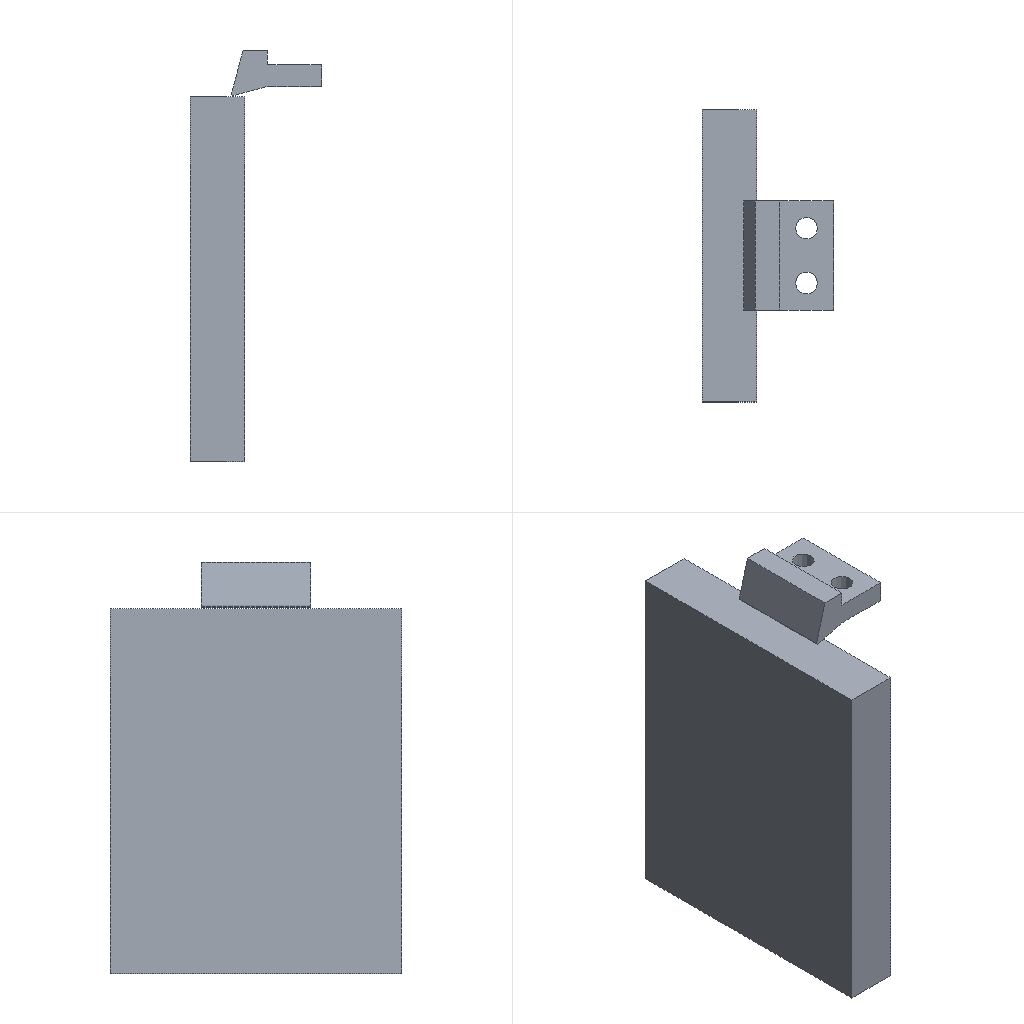Simulation study | abaqus
Set-up summary:
category,name,step,type,value,unit,region
solver,abaqus
solver,version,,,Abaqus/Explicit 2020
units,not stated in the deck,,not stated
analysis,deck,,transient,transient
load_step,Step-1,Step-1,transient
load_step,requested,,,1
mesh,nodes,,,255942
mesh,elements,,,232218
element_type,C3D8,,solid,3738
element_type,C3D8R,,solid,228480
load,load commands in deck,,count,1
bc,support commands in deck,,count,7
material,Q345,,in results
material,SLPSB,,in results
material,SLPSB2,,in results
material,SOIL,,in results
material,SOIL-COPY,,in results
check,setup vs results,,match,"per instance, exact: element labels, types and connectivity; labels of the nodes the elements use; coordinates not compared"
Abaqus input file, long lists of numbers shortened:
*Heading
** Job name:  Model name: Model-1
** Generated by: Abaqus/CAE 2020
*Preprint, echo=NO, model=NO, history=NO, contact=NO
**
** PARTS
**
*Part, name=newwork
*Node
      1,          10.,           0.,        -100.
      2,          15.,           0.,        -100.
** (251158 more lines like these left out)
*Element, type=C3D8R
     1,   1043,  31614,  69742,   6018,      1,     41,   3333,    136
     2,  31614,  31615,  69743,  69742,     41,     42,   3334,   3333
** (228478 more lines like these left out)
*Nset, nset=Set-31
      9,     10,     13,     14,     15,     16,     19,     20,     35,     36,     37,     38,    398,    399,    400,    401
    402,    403,    404,    405,    406,    407,    408,    409,    410,    411,    412,    413,    414,    415,    416,    417
** (632 more lines like these left out)
*Elset, elset=Set-31, generate
 216641,  223040,       1
*Nset, nset=Set-32
      1,      2,      3,      4,      5,      6,      7,      8,      9,     10,     11,     12,     13,     14,     15,     16
     17,     18,     19,     20,     21,     22,     23,     24,     25,     26,     27,     28,     29,     30,     31,     32
** (15314 more lines like these left out)
*Elset, elset=Set-32
      1,      2,      3,      4,      5,      6,      7,      8,      9,     10,     11,     12,     13,     14,     15,     16
     17,     18,     19,     20,     21,     22,     23,     24,     25,     26,     27,     28,     29,     30,     31,     32
** (13878 more lines like these left out)
*Nset, nset=chipquanchip
      3,      4,      5,      6,     13,     14,     28,     29,     31,     32,     35,     36,     76,     77,     78,     79
     80,     81,     82,     83,     84,     85,     86,     87,     88,     89,     90,     91,     92,     93,     94,     95
** (8661 more lines like these left out)
*Elset, elset=zishiying
    371,    372,    373,    374,    375,    376,    377,    378,    379,    381,    382,    383,    384,    385,    386,    387
    388,    389,    390,    391,    392,    393,    394,    395,    396,    397,    398,    399,    400,    401,    402,    403
** (6313 more lines like these left out)
** Section: tu
*Solid Section, elset=Set-32, material=soil
,
** Section: suliao
*Solid Section, elset=Set-31, material=slpsb
,
*End Part
**
*Part, name=qiedao
*Node
      1,           3.,   7.052,           0.
      2,          -3.,   7.052,           0.
** (4779 more lines like these left out)
*Element, type=C3D8
   1,  408,  428,  429,  410, 2071, 2091, 2092, 2073
   2,   42,   41,    5,    6, 1026, 1027,  196,  138
** (3736 more lines like these left out)
*Node
   4782, 1.55431223e-15,   7.052,          15.
*Nset, nset=qiedao-RefPt_, internal
4782,
*Nset, nset=_PickedSet2, internal, generate
    1,  4781,     1
*Elset, elset=_PickedSet2, internal, generate
    1,  3738,     1
*Nset, nset=Set-daoju, generate
    1,  4782,     1
*Elset, elset=Set-daoju, generate
    1,  3738,     1
*Elset, elset=ganggang
    1,    2,    3,    4,    5,    6,    7,    8,    9,   10,   11,   12,   13,   14,   15,   16
   17,   18,   19,   20,   21,   22,   23,   24,   25,   26,   27,   28,   29,   30,   31,   32
** (104 more lines like these left out)
*Elset, elset=_keng-dao_S1, internal
    1,    2,    3,    4,    5,    6,    7,    8,    9,   10,   11,   12,   13,   14,   15,   16
   17,   18,   19,   20,   21,   22,   23,   24,   25,   26,   27,   28,   29,   30,   31,   32
** (22 more lines like these left out)
*Elset, elset=_keng-dao_S2, internal
 2524, 2525, 2526, 2527, 2528, 2529, 2530, 2531, 2532, 2533, 2534, 2535, 2536, 2537, 2538, 2539
 2540, 2541, 2542, 2543, 2544, 2545, 2546, 2547, 2548, 2549, 2550, 2551, 2552, 2553, 2554, 2555
** (22 more lines like these left out)
*Elset, elset=_keng-dao_S3, internal
    2,    5,    7,   10,   11,   12,   13,   16,   18,   21,   27,   28,   36,   89,   92,   94
   97,   98,   99,  100,  103,  105,  108,  114,  115,  123,  176,  179,  181,  184,  185,  186
** (29 more lines like these left out)
*Elset, elset=_keng-dao_S4, internal
    2,   89,  176,  263,  350,  437,  524,  611,  698,  785,  872,  959, 1046, 1133, 1220, 1307
 1394, 1481, 1568, 1655, 1742, 1829, 1916, 2003, 2090, 2177, 2264, 2351, 2438, 2525, 2640, 2722
** (3 more lines like these left out)
*Elset, elset=_keng-dao_S5, internal
    3,    8,   14,   15,   17,   19,   25,   29,   30,   31,   39,   41,   42,   44,   90,   95
  101,  102,  104,  106,  112,  116,  117,  118,  126,  128,  129,  131,  177,  182,  188,  189
** (30 more lines like these left out)
*Elset, elset=_keng-dao_S6, internal
    2,    8,   22,   84,   89,   95,  109,  171,  176,  182,  196,  258,  263,  269,  283,  345
  350,  356,  370,  432,  437,  443,  457,  519,  524,  530,  544,  606,  611,  617,  631,  693
** (9 more lines like these left out)
*Surface, type=ELEMENT, name=keng-dao
_keng-dao_S1, S1
_keng-dao_S2, S2
_keng-dao_S4, S4
_keng-dao_S6, S6
_keng-dao_S3, S3
_keng-dao_S5, S5
** Section: Q345
*Solid Section, elset=_PickedSet2, material=q345
,
*End Part
**
**
** ASSEMBLY
**
*Assembly, name=Assembly
**
*Instance, name=newwork-1, part=newwork
*End Instance
**
*Instance, name=qiedao-1, part=qiedao
   28.199,         -55., 5.826
   28.199,         -55., 5.826, 27.621, -54.423, 6.403,         120.
*End Instance
**
*Nset, nset=Set-20, instance=qiedao-1
 4782,
*Nset, nset=Set-22, instance=newwork-1
    21,    22,    23,    24,    25,    26,    39,    40,  1776,  1777,  1778,  1779,  1780,  1781,  1782,  1783
  1784,  1785,  1786,  1787,  1788,  1789,  1790,  1791,  1792,  1793,  1794,  1795,  1796,  1797,  1798,  1799
** (1206 more lines like these left out)
*Elset, elset=Set-22, instance=newwork-1
 169921, 169922, 169923, 169924, 169925, 169926, 169927, 169928, 169929, 169930, 169931, 169932, 169933, 169934, 169935, 169936
 169937, 169938, 169939, 169940, 169941, 169942, 169943, 169944, 169945, 169946, 169947, 169948, 169949, 169950, 169951, 169952
** (1188 more lines like these left out)
*Nset, nset=Set-23, instance=newwork-1
     1,     2,     7,     8,     9,    10,    11,    12,    15,    16,    17,    18,    19,    20,    21,    22
    23,    24,    25,    26,    27,    30,    33,    34,    37,    38,    39,    40,    41,    42,    43,    44
** (193 more lines like these left out)
*Elset, elset=Set-23, instance=newwork-1
      1,      2,      3,      4,      5,      6,      7,      8,      9,     10,   1591,   1592,   1593,   1594,   1595,   1596
   1597,   1598,   1599,   1600,   1601,   1602,   1603,   1604,   1605,   1606,   1607,   1608,   1609,   1610,   3191,   3192
** (177 more lines like these left out)
*Nset, nset=Set-24, instance=newwork-1
    19,    20,    35,    36,    37,    38,  1565,  1566,  1567,  1568,  1569,  1570,  1571,  1572,  1573,  1574
  1575,  1576,  1577,  1578,  1579,  1580,  1581,  1582,  1583,  1584,  1585,  1586,  1587,  1588,  1589,  1590
** (29 more lines like these left out)
*Elset, elset=Set-24, instance=newwork-1
 216321, 216322, 216323, 216324, 216325, 216326, 216327, 216328, 216329, 216330, 216331, 216332, 216333, 216334, 216335, 216336
 216337, 216338, 216339, 216340, 216341, 216342, 216343, 216344, 216345, 216346, 216347, 216348, 216349, 216350, 216351, 216352
** (38 more lines like these left out)
*Nset, nset=_PickedSet56, internal, instance=qiedao-1
 4782,
*Nset, nset=_PickedSet60, internal, instance=newwork-1
      1,      2,      3,      4,      5,      6,      7,      8,      9,     10,     11,     12,     13,     14,     15,     16
     17,     18,     19,     20,     27,     28,     29,     30,     31,     32,     33,     34,     35,     36,     37,     38
** (13281 more lines like these left out)
*Elset, elset=_PickedSet60, internal, instance=newwork-1
      1,      2,      3,      4,      5,      6,      7,      8,      9,     10,     11,     12,     13,     14,     15,     16
     17,     18,     19,     20,     21,     22,     23,     24,     25,     26,     27,     28,     29,     30,     31,     32
** (11898 more lines like these left out)
*Surface, type=NODE, name=newwork-1_chipquanchip_CNS_, internal
newwork-1.chipquanchip, 1.
** Constraint: Constraint-1
*Rigid Body, ref node=_PickedSet56, elset=qiedao-1.ganggang
*End Assembly
**
** MATERIALS
**
*Material, name=q345
*Density
 7.85e-09,
*Elastic
206000., 0.3
*Material, name=slpsb
*Damage Initiation, criterion=SHEAR
 0.007,0.,0.
*Damage Evolution, type=DISPLACEMENT
 2e-05,
*Density
 1.2e-09,
*Elastic
890000., 0.42
*Plastic
   0.001,        0.
 19.066,  0.02392
 29.961, 0.03986
 38.132, 0.05393
 49.027, 0.07081
 100.778, 0.09335
 147.082,   0.1084
 198.833,  0.1192
 242.412,  0.1277
 299.611,  0.1357
 345.914,  0.1423
 397.665,  0.1479
 446.693,  0.1559
  495.72,  0.1639
 542.023,  0.1691
 593.774,  0.1748
*Material, name=slpsb2
*Damage Initiation, criterion=SHEAR
 0.5,   0.33, 0.0001
*Damage Evolution, type=DISPLACEMENT
 0.5,
*Density
 1.88e-09,
*Elastic
 10.9, 0.35
*Plastic
   0.001,        0.
 19.066,  0.02392
 29.961, 0.03986
 38.132, 0.05393
 49.027, 0.07081
 100.778, 0.09335
 147.082,   0.1084
 198.833,  0.1192
 242.412,  0.1277
 299.611,  0.1357
 345.914,  0.1423
 397.665,  0.1479
 446.693,  0.1559
  495.72,  0.1639
 542.023,  0.1691
 593.774,  0.1748
*Material, name=soil
*Damage Initiation, criterion=SHEAR
 0.007,0.,0.
*Damage Evolution, type=DISPLACEMENT
 0.007,
*Density
 1.88e-09,
*Drucker Prager
35., 0.885,   29.
*Drucker Prager Hardening
10.,0.
*Elastic
 10.9, 0.35
*Material, name=soil-Copy
*Damage Initiation, criterion=SHEAR
 0.5,   0.33, 0.0001
*Damage Evolution, type=DISPLACEMENT
 0.03,
*Density
 1.88e-09,
*Elastic
 10.9, 0.35
*Plastic
 9.,   0.
12., 0.02
15., 0.04
17., 0.06
18., 0.08
19.,  0.1
20., 0.12
**
** INTERACTION PROPERTIES
**
*Surface Interaction, name=IntProp-1
*Friction
 0.3,
*Surface Behavior, pressure-overclosure=HARD
**
** BOUNDARY CONDITIONS
**
** Name: BC-7 Type: 对称/反对称/完全固定
*Boundary
Set-22, ENCASTRE
** ----------------------------------------------------------------
**
** STEP: Step-1
**
*Step, name=Step-1, nlgeom=YES
*Dynamic, Explicit
, 1.6
*Bulk Viscosity
0.06, 1.2
** Mass Scaling: Semi-Automatic
**               Whole Model
*Fixed Mass Scaling, dt=1e-05, type=below min
**
** BOUNDARY CONDITIONS
**
** Name: jingei Type: Velocity/Angular velocity
*Boundary, type=VELOCITY
Set-20, 1, 1
Set-20, 2, 2
Set-20, 3, 3, -30.
Set-20, 4, 4
Set-20, 5, 5
Set-20, 6, 6
*Adaptive Mesh Controls, name=Ada-1
1., 0., 0.
**
** INTERACTIONS
**
** Interaction: Int-1
*Contact Pair, interaction=IntProp-1, mechanical constraint=KINEMATIC, cpset=Int-1
qiedao-1.keng-dao, newwork-1_chipquanchip_CNS_
**
** OUTPUT REQUESTS
**
*Restart, write, number interval=1, time marks=NO
**
** FIELD OUTPUT: F-Output-1
**
*Output, field, number interval=200
*Node Output
A, RF, RT, U, V
*Element Output, directions=YES
LE, MISES, PE, PEEQ, PEEQVAVG, PEVAVG, S, STATUS
*Contact Output
CSTRESS,
**
** HISTORY OUTPUT: H-Output-1
**
*Output, history, variable=PRESELECT
*End Step
Results summary:
result,step,Step-1,partial,increments=15136 time=0.1144/1.6
result,analysis,,,transient
result,last_loadstep,,,1
result,primary field,,,U
result,reaction total,,FX,2.434,model units
result,reaction total,,FY,-4.463,model units
result,reaction total,,FZ,-247.791,model units